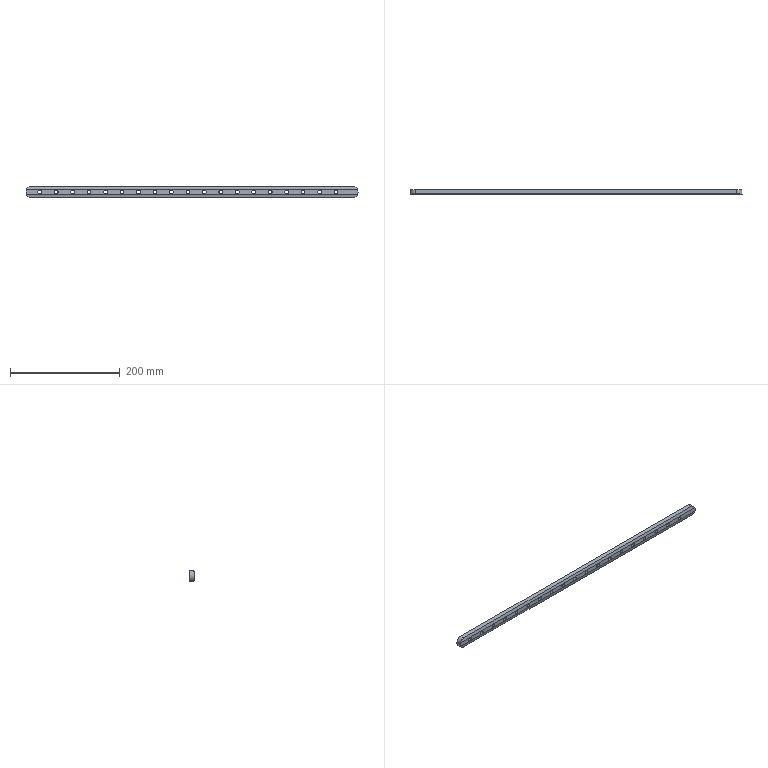Part | SolidWorks | features Chamfer 1, Extrusion 1, HoleWzd 1, ICE 1, LPattern 1 | 1 solid | 46 faces | box 605 x 9 x 20 mm | volume 97161 mm3 | cylinder 40 | plane 6 | commonest cylinder face diameters 6.8 x38 20 x2